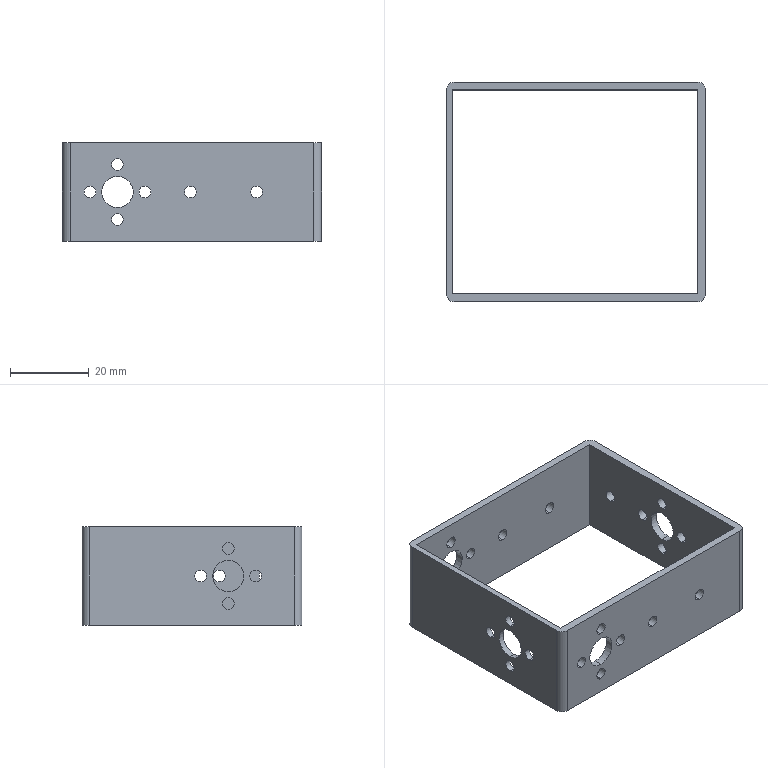Part | SolidWorks | features ICE 5, Fillet 2, Extrusion 1, MirrorPattern 1 | 1 solid | 66 faces | box 66 x 56 x 25 mm | volume 10390 mm3 | cylinder 56 | plane 10 | commonest cylinder face diameters 3 x44 8 x8 4 x4